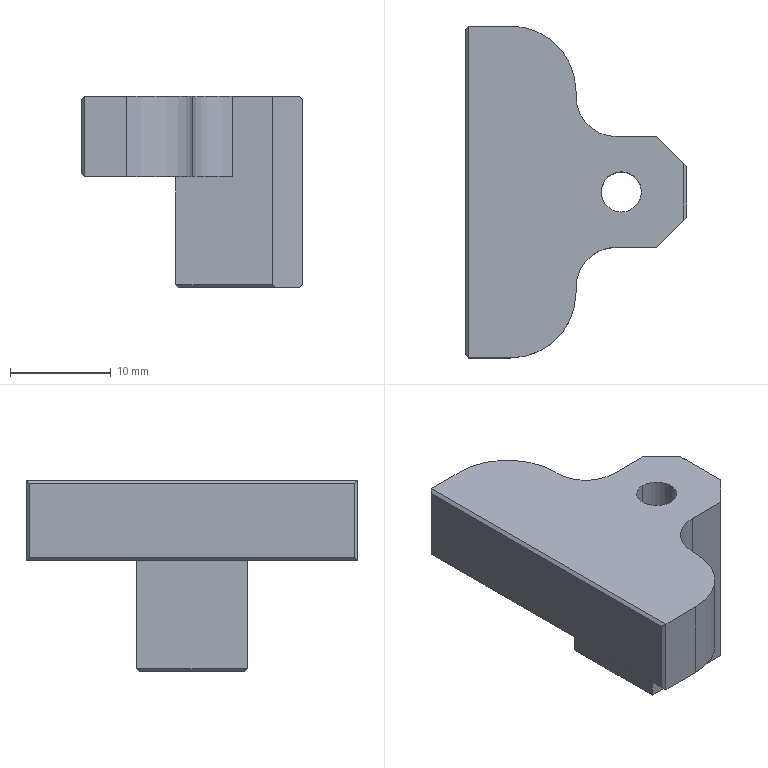Part | NX | 1 solid | 37 faces | box 22 x 33 x 19 mm | volume 4850 mm3 | plane 23 | cylinder 10 | cone 4 | commonest cylinder face diameters 2.5 x4 4 x2 8 x2 13 x2